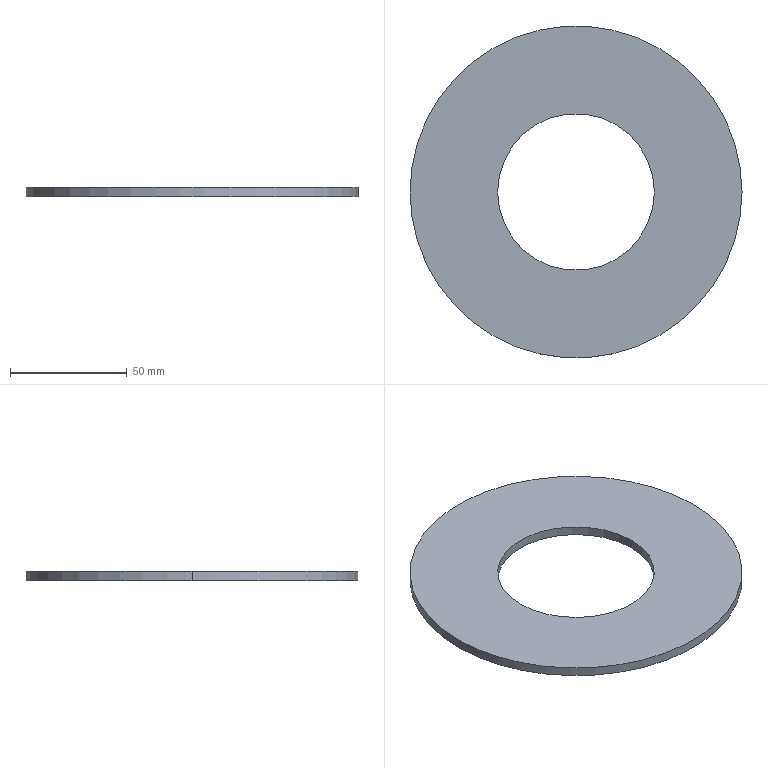Part | NX | features BREP 1 | 1 solid | 6 faces | box 142 x 142 x 4 mm | volume 49244 mm3 | cylinder 4 | plane 2 | commonest cylinder face diameters 67 x2 142 x2
STEP:
#1=CARTESIAN_POINT('',(-33.5,0.,4.));
#2=VERTEX_POINT('',#1);
#3=CARTESIAN_POINT('',(33.5,0.,4.));
#4=VERTEX_POINT('',#3);
#5=CARTESIAN_POINT('',(0.,0.,4.));
#6=DIRECTION('',(0.,0.,1.));
#7=DIRECTION('',(1.,0.,0.));
#8=AXIS2_PLACEMENT_3D('',#5,#6,#7);
#9=CIRCLE('',#8,33.5);
#10=EDGE_CURVE('',#2,#4,#9,.T.);
#11=ORIENTED_EDGE('',*,*,#10,.T.);
#12=CARTESIAN_POINT('',(33.5,0.,0.));
#13=VERTEX_POINT('',#12);
#14=CARTESIAN_POINT('',(33.5,0.,4.));
#15=DIRECTION('',(0.,0.,-1.));
#16=VECTOR('',#15,1000.);
#17=LINE('',#14,#16);
#18=EDGE_CURVE('',#13,#4,#17,.F.);
#19=ORIENTED_EDGE('',*,*,#18,.F.);
#20=CARTESIAN_POINT('',(-33.5,0.,0.));
#21=VERTEX_POINT('',#20);
#22=CARTESIAN_POINT('',(0.,0.,0.));
#23=DIRECTION('',(0.,0.,1.));
#24=DIRECTION('',(1.,0.,0.));
#25=AXIS2_PLACEMENT_3D('',#22,#23,#24);
#26=CIRCLE('',#25,33.5);
#27=EDGE_CURVE('',#21,#13,#26,.T.);
#28=ORIENTED_EDGE('',*,*,#27,.F.);
#29=CARTESIAN_POINT('',(-33.5,0.,4.));
#30=DIRECTION('',(0.,0.,-1.));
#31=VECTOR('',#30,1000.);
#32=LINE('',#29,#31);
#33=EDGE_CURVE('',#21,#2,#32,.F.);
#34=ORIENTED_EDGE('',*,*,#33,.T.);
#35=EDGE_LOOP('',(#11,#19,#28,#34));
#36=FACE_BOUND('',#35,.T.);
#37=CARTESIAN_POINT('',(0.,0.,4.));
#38=DIRECTION('',(0.,0.,-1.));
#39=DIRECTION('',(1.,0.,0.));
#40=AXIS2_PLACEMENT_3D('',#37,#38,#39);
#41=CYLINDRICAL_SURFACE('',#40,33.5);
#42=ADVANCED_FACE('',(#36),#41,.F.);
#43=CARTESIAN_POINT('',(71.,0.,4.));
#44=VERTEX_POINT('',#43);
#45=CARTESIAN_POINT('',(-71.,0.,4.));
#46=VERTEX_POINT('',#45);
#47=CARTESIAN_POINT('',(0.,0.,4.));
#48=DIRECTION('',(0.,0.,1.));
#49=DIRECTION('',(1.,0.,0.));
#50=AXIS2_PLACEMENT_3D('',#47,#48,#49);
#51=CIRCLE('',#50,71.);
#52=EDGE_CURVE('',#44,#46,#51,.T.);
#53=ORIENTED_EDGE('',*,*,#52,.F.);
#54=CARTESIAN_POINT('',(71.,0.,0.));
#55=VERTEX_POINT('',#54);
#56=CARTESIAN_POINT('',(71.,0.,4.));
#57=DIRECTION('',(0.,0.,-1.));
#58=VECTOR('',#57,1000.);
#59=LINE('',#56,#58);
#60=EDGE_CURVE('',#55,#44,#59,.F.);
#61=ORIENTED_EDGE('',*,*,#60,.F.);
#62=CARTESIAN_POINT('',(-71.,0.,0.));
#63=VERTEX_POINT('',#62);
#64=CARTESIAN_POINT('',(0.,0.,0.));
#65=DIRECTION('',(0.,0.,1.));
#66=DIRECTION('',(1.,0.,0.));
#67=AXIS2_PLACEMENT_3D('',#64,#65,#66);
#68=CIRCLE('',#67,71.);
#69=EDGE_CURVE('',#55,#63,#68,.T.);
#70=ORIENTED_EDGE('',*,*,#69,.T.);
#71=CARTESIAN_POINT('',(-71.,0.,4.));
#72=DIRECTION('',(0.,0.,-1.));
#73=VECTOR('',#72,1000.);
#74=LINE('',#71,#73);
#75=EDGE_CURVE('',#63,#46,#74,.F.);
#76=ORIENTED_EDGE('',*,*,#75,.T.);
#77=EDGE_LOOP('',(#53,#61,#70,#76));
#78=FACE_BOUND('',#77,.T.);
#79=CARTESIAN_POINT('',(0.,0.,4.));
#80=DIRECTION('',(0.,0.,-1.));
#81=DIRECTION('',(1.,0.,0.));
#82=AXIS2_PLACEMENT_3D('',#79,#80,#81);
#83=CYLINDRICAL_SURFACE('',#82,71.);
#84=ADVANCED_FACE('',(#78),#83,.T.);
#85=CARTESIAN_POINT('',(0.,0.,4.));
#86=DIRECTION('',(0.,0.,1.));
#87=DIRECTION('',(1.,0.,0.));
#88=AXIS2_PLACEMENT_3D('',#85,#86,#87);
#89=CIRCLE('',#88,71.);
#90=EDGE_CURVE('',#46,#44,#89,.T.);
#91=ORIENTED_EDGE('',*,*,#90,.T.);
#92=ORIENTED_EDGE('',*,*,#52,.T.);
#93=EDGE_LOOP('',(#91,#92));
#94=FACE_BOUND('',#93,.T.);
#95=ORIENTED_EDGE('',*,*,#10,.F.);
#96=CARTESIAN_POINT('',(0.,0.,4.));
#97=DIRECTION('',(0.,0.,1.));
#98=DIRECTION('',(1.,0.,0.));
#99=AXIS2_PLACEMENT_3D('',#96,#97,#98);
#100=CIRCLE('',#99,33.5);
#101=EDGE_CURVE('',#4,#2,#100,.T.);
#102=ORIENTED_EDGE('',*,*,#101,.F.);
#103=EDGE_LOOP('',(#95,#102));
#104=FACE_BOUND('',#103,.T.);
#105=CARTESIAN_POINT('',(0.,0.,4.));
#106=DIRECTION('',(0.,0.,1.));
#107=DIRECTION('',(-1.,0.,0.));
#108=AXIS2_PLACEMENT_3D('',#105,#106,#107);
#109=PLANE('',#108);
#110=ADVANCED_FACE('',(#94,#104),#109,.T.);
#111=CARTESIAN_POINT('',(0.,0.,0.));
#112=DIRECTION('',(0.,0.,1.));
#113=DIRECTION('',(1.,0.,0.));
#114=AXIS2_PLACEMENT_3D('',#111,#112,#113);
#115=CIRCLE('',#114,71.);
#116=EDGE_CURVE('',#63,#55,#115,.T.);
#117=ORIENTED_EDGE('',*,*,#116,.F.);
#118=ORIENTED_EDGE('',*,*,#69,.F.);
#119=EDGE_LOOP('',(#117,#118));
#120=FACE_BOUND('',#119,.T.);
#121=ORIENTED_EDGE('',*,*,#27,.T.);
#122=CARTESIAN_POINT('',(0.,0.,0.));
#123=DIRECTION('',(0.,0.,1.));
#124=DIRECTION('',(1.,0.,0.));
#125=AXIS2_PLACEMENT_3D('',#122,#123,#124);
#126=CIRCLE('',#125,33.5);
#127=EDGE_CURVE('',#13,#21,#126,.T.);
#128=ORIENTED_EDGE('',*,*,#127,.T.);
#129=EDGE_LOOP('',(#121,#128));
#130=FACE_BOUND('',#129,.T.);
#131=CARTESIAN_POINT('',(0.,0.,0.));
#132=DIRECTION('',(0.,0.,1.));
#133=DIRECTION('',(-1.,0.,0.));
#134=AXIS2_PLACEMENT_3D('',#131,#132,#133);
#135=PLANE('',#134);
#136=ADVANCED_FACE('',(#120,#130),#135,.F.);
#137=ORIENTED_EDGE('',*,*,#60,.T.);
#138=ORIENTED_EDGE('',*,*,#90,.F.);
#139=ORIENTED_EDGE('',*,*,#75,.F.);
#140=ORIENTED_EDGE('',*,*,#116,.T.);
#141=EDGE_LOOP('',(#137,#138,#139,#140));
#142=FACE_BOUND('',#141,.T.);
#143=CARTESIAN_POINT('',(0.,0.,4.));
#144=DIRECTION('',(0.,0.,-1.));
#145=DIRECTION('',(1.,0.,0.));
#146=AXIS2_PLACEMENT_3D('',#143,#144,#145);
#147=CYLINDRICAL_SURFACE('',#146,71.);
#148=ADVANCED_FACE('',(#142),#147,.T.);
#149=ORIENTED_EDGE('',*,*,#18,.T.);
#150=ORIENTED_EDGE('',*,*,#101,.T.);
#151=ORIENTED_EDGE('',*,*,#33,.F.);
#152=ORIENTED_EDGE('',*,*,#127,.F.);
#153=EDGE_LOOP('',(#149,#150,#151,#152));
#154=FACE_BOUND('',#153,.T.);
#155=CARTESIAN_POINT('',(0.,0.,4.));
#156=DIRECTION('',(0.,0.,-1.));
#157=DIRECTION('',(1.,0.,0.));
#158=AXIS2_PLACEMENT_3D('',#155,#156,#157);
#159=CYLINDRICAL_SURFACE('',#158,33.5);
#160=ADVANCED_FACE('',(#154),#159,.F.);
#161=CLOSED_SHELL('',(#42,#84,#110,#136,#148,#160));
#162=MANIFOLD_SOLID_BREP('',#161);
#163=(LENGTH_UNIT()NAMED_UNIT(*)SI_UNIT(.MILLI.,.METRE.));
#164=UNCERTAINTY_MEASURE_WITH_UNIT(LENGTH_MEASURE(0.00001),#163,'','');
#165=(NAMED_UNIT(*)PLANE_ANGLE_UNIT()SI_UNIT($,.RADIAN.));
#166=(NAMED_UNIT(*)SI_UNIT($,.STERADIAN.)SOLID_ANGLE_UNIT());
#167=(GEOMETRIC_REPRESENTATION_CONTEXT(3)GLOBAL_UNCERTAINTY_ASSIGNED_CONTEXT((#164))GLOBAL_UNIT_ASSIGNED_CONTEXT((#163,#165,#166))REPRESENTATION_CONTEXT('',''));
#168=ADVANCED_BREP_SHAPE_REPRESENTATION('',(#162),#167);